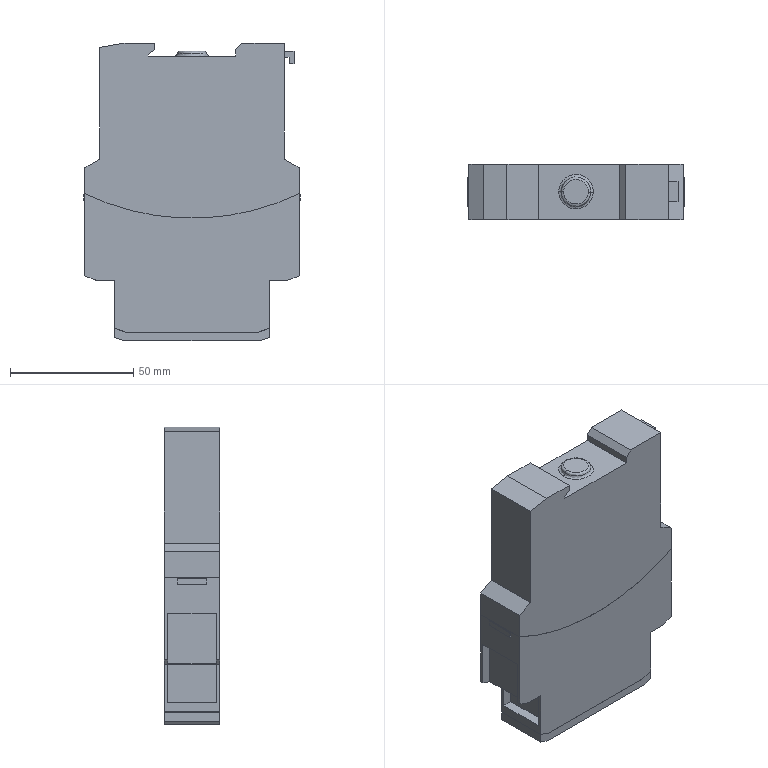Part | STEP file | PILZ safety relay PNOZX2 | 1 solid | 119 faces | box 87.8 x 22.5 x 120.6 mm | volume 199420 mm3 | plane 109 | cylinder 6 | spline 4 | commonest cylinder face diameters 0.865 x2 200 x2 1.73 x1 2.883 x1